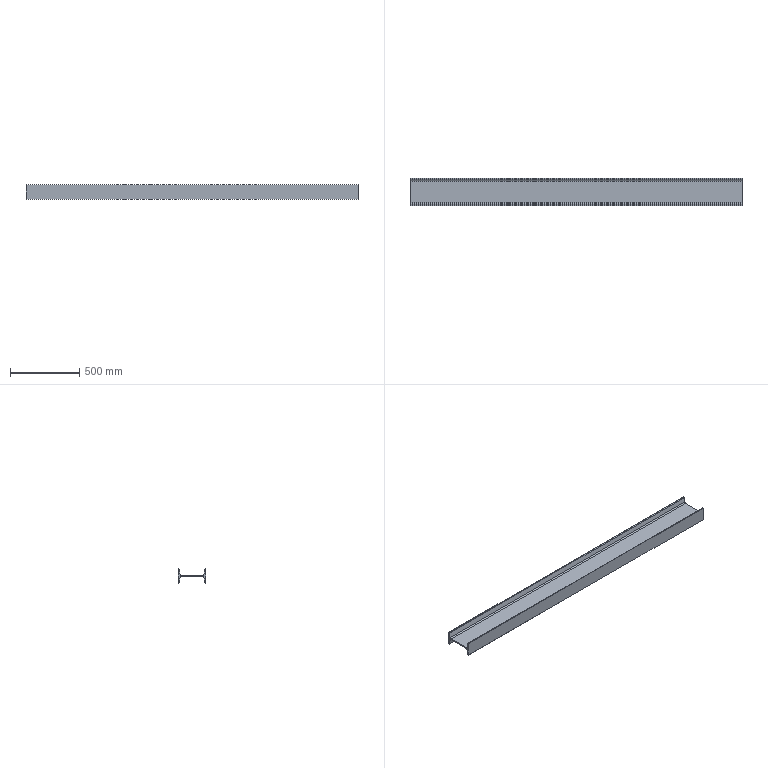Part | SolidWorks | features Fillet 2, Extrusion 1 | 1 solid | 22 faces | box 2400 x 200 x 102 mm | volume 9158318 mm3 | plane 14 | cylinder 8 | commonest cylinder face diameters 9 x4 18 x4
STEP:
#1=CARTESIAN_POINT('',(2400.,2.963,51.));
#2=VERTEX_POINT('',#1);
#3=CARTESIAN_POINT('',(2400.,0.,51.));
#4=VERTEX_POINT('',#3);
#5=CARTESIAN_POINT('',(2400.,6.775,51.));
#6=DIRECTION('',(0.,-1.,0.));
#7=VECTOR('',#6,1000.);
#8=LINE('',#5,#7);
#9=EDGE_CURVE('',#2,#4,#8,.T.);
#10=ORIENTED_EDGE('',*,*,#9,.F.);
#11=CARTESIAN_POINT('',(0.,2.963,51.));
#12=VERTEX_POINT('',#11);
#13=CARTESIAN_POINT('',(2400.,2.963,51.));
#14=DIRECTION('',(-1.,0.,0.));
#15=VECTOR('',#14,1000.);
#16=LINE('',#13,#15);
#17=EDGE_CURVE('',#2,#12,#16,.T.);
#18=ORIENTED_EDGE('',*,*,#17,.T.);
#19=CARTESIAN_POINT('',(0.,0.,51.));
#20=VERTEX_POINT('',#19);
#21=CARTESIAN_POINT('',(0.,6.775,51.));
#22=DIRECTION('',(0.,-1.,0.));
#23=VECTOR('',#22,1000.);
#24=LINE('',#21,#23);
#25=EDGE_CURVE('',#12,#20,#24,.T.);
#26=ORIENTED_EDGE('',*,*,#25,.T.);
#27=CARTESIAN_POINT('',(2400.,0.,51.));
#28=DIRECTION('',(-1.,0.,0.));
#29=VECTOR('',#28,1000.);
#30=LINE('',#27,#29);
#31=EDGE_CURVE('',#4,#20,#30,.T.);
#32=ORIENTED_EDGE('',*,*,#31,.F.);
#33=EDGE_LOOP('',(#10,#18,#26,#32));
#34=FACE_OUTER_BOUND('',#33,.T.);
#35=CARTESIAN_POINT('',(2400.,6.775,51.));
#36=DIRECTION('',(0.,0.,-1.));
#37=DIRECTION('',(-1.,0.,0.));
#38=AXIS2_PLACEMENT_3D('',#35,#36,#37);
#39=PLANE('',#38);
#40=ADVANCED_FACE('',(#34),#39,.F.);
#41=CARTESIAN_POINT('',(0.,0.,-51.));
#42=VERTEX_POINT('',#41);
#43=CARTESIAN_POINT('',(0.,0.,51.));
#44=DIRECTION('',(0.,0.,-1.));
#45=VECTOR('',#44,1000.);
#46=LINE('',#43,#45);
#47=EDGE_CURVE('',#20,#42,#46,.T.);
#48=ORIENTED_EDGE('',*,*,#47,.T.);
#49=CARTESIAN_POINT('',(2400.,0.,-51.));
#50=VERTEX_POINT('',#49);
#51=CARTESIAN_POINT('',(2400.,0.,-51.));
#52=DIRECTION('',(-1.,0.,0.));
#53=VECTOR('',#52,1000.);
#54=LINE('',#51,#53);
#55=EDGE_CURVE('',#50,#42,#54,.T.);
#56=ORIENTED_EDGE('',*,*,#55,.F.);
#57=CARTESIAN_POINT('',(2400.,0.,51.));
#58=DIRECTION('',(0.,0.,-1.));
#59=VECTOR('',#58,1000.);
#60=LINE('',#57,#59);
#61=EDGE_CURVE('',#4,#50,#60,.T.);
#62=ORIENTED_EDGE('',*,*,#61,.F.);
#63=ORIENTED_EDGE('',*,*,#31,.T.);
#64=EDGE_LOOP('',(#48,#56,#62,#63));
#65=FACE_OUTER_BOUND('',#64,.T.);
#66=CARTESIAN_POINT('',(2400.,0.,51.));
#67=DIRECTION('',(0.,1.,0.));
#68=DIRECTION('',(0.,0.,1.));
#69=AXIS2_PLACEMENT_3D('',#66,#67,#68);
#70=PLANE('',#69);
#71=ADVANCED_FACE('',(#65),#70,.F.);
#72=CARTESIAN_POINT('',(0.,2.963,-51.));
#73=VERTEX_POINT('',#72);
#74=CARTESIAN_POINT('',(0.,6.775,-51.));
#75=DIRECTION('',(0.,1.,0.));
#76=VECTOR('',#75,1000.);
#77=LINE('',#74,#76);
#78=EDGE_CURVE('',#42,#73,#77,.T.);
#79=ORIENTED_EDGE('',*,*,#78,.T.);
#80=CARTESIAN_POINT('',(2400.,2.963,-51.));
#81=VERTEX_POINT('',#80);
#82=CARTESIAN_POINT('',(2400.,2.963,-51.));
#83=DIRECTION('',(1.,0.,0.));
#84=VECTOR('',#83,1000.);
#85=LINE('',#82,#84);
#86=EDGE_CURVE('',#73,#81,#85,.T.);
#87=ORIENTED_EDGE('',*,*,#86,.T.);
#88=CARTESIAN_POINT('',(2400.,6.775,-51.));
#89=DIRECTION('',(0.,1.,0.));
#90=VECTOR('',#89,1000.);
#91=LINE('',#88,#90);
#92=EDGE_CURVE('',#50,#81,#91,.T.);
#93=ORIENTED_EDGE('',*,*,#92,.F.);
#94=ORIENTED_EDGE('',*,*,#55,.T.);
#95=EDGE_LOOP('',(#79,#87,#93,#94));
#96=FACE_OUTER_BOUND('',#95,.T.);
#97=CARTESIAN_POINT('',(2400.,6.775,-51.));
#98=DIRECTION('',(0.,0.,1.));
#99=DIRECTION('',(1.,0.,0.));
#100=AXIS2_PLACEMENT_3D('',#97,#98,#99);
#101=PLANE('',#100);
#102=ADVANCED_FACE('',(#96),#101,.F.);
#103=CARTESIAN_POINT('',(2400.,7.402,-47.24));
#104=VERTEX_POINT('',#103);
#105=CARTESIAN_POINT('',(2400.,13.272,-12.02));
#106=VERTEX_POINT('',#105);
#107=CARTESIAN_POINT('',(2400.,14.525,-4.5));
#108=DIRECTION('',(0.,0.1644,0.9864));
#109=VECTOR('',#108,1000.);
#110=LINE('',#107,#109);
#111=EDGE_CURVE('',#104,#106,#110,.T.);
#112=ORIENTED_EDGE('',*,*,#111,.F.);
#113=CARTESIAN_POINT('',(0.,7.402,-47.24));
#114=VERTEX_POINT('',#113);
#115=CARTESIAN_POINT('',(2400.,7.402,-47.24));
#116=DIRECTION('',(-1.,0.,0.));
#117=VECTOR('',#116,1000.);
#118=LINE('',#115,#117);
#119=EDGE_CURVE('',#104,#114,#118,.T.);
#120=ORIENTED_EDGE('',*,*,#119,.T.);
#121=CARTESIAN_POINT('',(0.,13.272,-12.02));
#122=VERTEX_POINT('',#121);
#123=CARTESIAN_POINT('',(0.,14.525,-4.5));
#124=DIRECTION('',(0.,0.1644,0.9864));
#125=VECTOR('',#124,1000.);
#126=LINE('',#123,#125);
#127=EDGE_CURVE('',#114,#122,#126,.T.);
#128=ORIENTED_EDGE('',*,*,#127,.T.);
#129=CARTESIAN_POINT('',(2400.,13.272,-12.02));
#130=DIRECTION('',(1.,0.,0.));
#131=VECTOR('',#130,1000.);
#132=LINE('',#129,#131);
#133=EDGE_CURVE('',#122,#106,#132,.T.);
#134=ORIENTED_EDGE('',*,*,#133,.T.);
#135=EDGE_LOOP('',(#112,#120,#128,#134));
#136=FACE_OUTER_BOUND('',#135,.T.);
#137=CARTESIAN_POINT('',(2400.,14.525,-4.5));
#138=DIRECTION('',(0.,-0.9864,0.1644));
#139=DIRECTION('',(0.,-0.1644,-0.9864));
#140=AXIS2_PLACEMENT_3D('',#137,#138,#139);
#141=PLANE('',#140);
#142=ADVANCED_FACE('',(#136),#141,.F.);
#143=CARTESIAN_POINT('',(0.,22.149,-4.5));
#144=VERTEX_POINT('',#143);
#145=CARTESIAN_POINT('',(0.,177.851,-4.5));
#146=VERTEX_POINT('',#145);
#147=CARTESIAN_POINT('',(0.,185.475,-4.5));
#148=DIRECTION('',(0.,1.,0.));
#149=VECTOR('',#148,1000.);
#150=LINE('',#147,#149);
#151=EDGE_CURVE('',#144,#146,#150,.T.);
#152=ORIENTED_EDGE('',*,*,#151,.T.);
#153=CARTESIAN_POINT('',(2400.,177.851,-4.5));
#154=VERTEX_POINT('',#153);
#155=CARTESIAN_POINT('',(2400.,177.851,-4.5));
#156=DIRECTION('',(1.,0.,0.));
#157=VECTOR('',#156,1000.);
#158=LINE('',#155,#157);
#159=EDGE_CURVE('',#146,#154,#158,.T.);
#160=ORIENTED_EDGE('',*,*,#159,.T.);
#161=CARTESIAN_POINT('',(2400.,22.149,-4.5));
#162=VERTEX_POINT('',#161);
#163=CARTESIAN_POINT('',(2400.,185.475,-4.5));
#164=DIRECTION('',(0.,1.,0.));
#165=VECTOR('',#164,1000.);
#166=LINE('',#163,#165);
#167=EDGE_CURVE('',#162,#154,#166,.T.);
#168=ORIENTED_EDGE('',*,*,#167,.F.);
#169=CARTESIAN_POINT('',(0.,22.149,-4.5));
#170=DIRECTION('',(-1.,0.,0.));
#171=VECTOR('',#170,1000.);
#172=LINE('',#169,#171);
#173=EDGE_CURVE('',#162,#144,#172,.T.);
#174=ORIENTED_EDGE('',*,*,#173,.T.);
#175=EDGE_LOOP('',(#152,#160,#168,#174));
#176=FACE_OUTER_BOUND('',#175,.T.);
#177=CARTESIAN_POINT('',(2400.,185.475,-4.5));
#178=DIRECTION('',(0.,0.,1.));
#179=DIRECTION('',(0.,-1.,0.));
#180=AXIS2_PLACEMENT_3D('',#177,#178,#179);
#181=PLANE('',#180);
#182=ADVANCED_FACE('',(#176),#181,.F.);
#183=CARTESIAN_POINT('',(0.,186.728,-12.02));
#184=VERTEX_POINT('',#183);
#185=CARTESIAN_POINT('',(0.,192.598,-47.24));
#186=VERTEX_POINT('',#185);
#187=CARTESIAN_POINT('',(0.,193.225,-51.));
#188=DIRECTION('',(0.,0.1644,-0.9864));
#189=VECTOR('',#188,1000.);
#190=LINE('',#187,#189);
#191=EDGE_CURVE('',#184,#186,#190,.T.);
#192=ORIENTED_EDGE('',*,*,#191,.T.);
#193=CARTESIAN_POINT('',(2400.,192.598,-47.24));
#194=VERTEX_POINT('',#193);
#195=CARTESIAN_POINT('',(2400.,192.598,-47.24));
#196=DIRECTION('',(1.,0.,0.));
#197=VECTOR('',#196,1000.);
#198=LINE('',#195,#197);
#199=EDGE_CURVE('',#186,#194,#198,.T.);
#200=ORIENTED_EDGE('',*,*,#199,.T.);
#201=CARTESIAN_POINT('',(2400.,186.728,-12.02));
#202=VERTEX_POINT('',#201);
#203=CARTESIAN_POINT('',(2400.,193.225,-51.));
#204=DIRECTION('',(0.,0.1644,-0.9864));
#205=VECTOR('',#204,1000.);
#206=LINE('',#203,#205);
#207=EDGE_CURVE('',#202,#194,#206,.T.);
#208=ORIENTED_EDGE('',*,*,#207,.F.);
#209=CARTESIAN_POINT('',(0.,186.728,-12.02));
#210=DIRECTION('',(-1.,0.,0.));
#211=VECTOR('',#210,1000.);
#212=LINE('',#209,#211);
#213=EDGE_CURVE('',#202,#184,#212,.T.);
#214=ORIENTED_EDGE('',*,*,#213,.T.);
#215=EDGE_LOOP('',(#192,#200,#208,#214));
#216=FACE_OUTER_BOUND('',#215,.T.);
#217=CARTESIAN_POINT('',(2400.,193.225,-51.));
#218=DIRECTION('',(0.,0.9864,0.1644));
#219=DIRECTION('',(0.,-0.1644,0.9864));
#220=AXIS2_PLACEMENT_3D('',#217,#218,#219);
#221=PLANE('',#220);
#222=ADVANCED_FACE('',(#216),#221,.F.);
#223=CARTESIAN_POINT('',(2400.,197.037,-51.));
#224=VERTEX_POINT('',#223);
#225=CARTESIAN_POINT('',(2400.,200.,-51.));
#226=VERTEX_POINT('',#225);
#227=CARTESIAN_POINT('',(2400.,200.,-51.));
#228=DIRECTION('',(0.,1.,0.));
#229=VECTOR('',#228,1000.);
#230=LINE('',#227,#229);
#231=EDGE_CURVE('',#224,#226,#230,.T.);
#232=ORIENTED_EDGE('',*,*,#231,.F.);
#233=CARTESIAN_POINT('',(0.,197.037,-51.));
#234=VERTEX_POINT('',#233);
#235=CARTESIAN_POINT('',(2400.,197.037,-51.));
#236=DIRECTION('',(-1.,0.,0.));
#237=VECTOR('',#236,1000.);
#238=LINE('',#235,#237);
#239=EDGE_CURVE('',#224,#234,#238,.T.);
#240=ORIENTED_EDGE('',*,*,#239,.T.);
#241=CARTESIAN_POINT('',(0.,200.,-51.));
#242=VERTEX_POINT('',#241);
#243=CARTESIAN_POINT('',(0.,200.,-51.));
#244=DIRECTION('',(0.,1.,0.));
#245=VECTOR('',#244,1000.);
#246=LINE('',#243,#245);
#247=EDGE_CURVE('',#234,#242,#246,.T.);
#248=ORIENTED_EDGE('',*,*,#247,.T.);
#249=CARTESIAN_POINT('',(2400.,200.,-51.));
#250=DIRECTION('',(-1.,0.,0.));
#251=VECTOR('',#250,1000.);
#252=LINE('',#249,#251);
#253=EDGE_CURVE('',#226,#242,#252,.T.);
#254=ORIENTED_EDGE('',*,*,#253,.F.);
#255=EDGE_LOOP('',(#232,#240,#248,#254));
#256=FACE_OUTER_BOUND('',#255,.T.);
#257=CARTESIAN_POINT('',(2400.,200.,-51.));
#258=DIRECTION('',(0.,0.,1.));
#259=DIRECTION('',(0.,-1.,0.));
#260=AXIS2_PLACEMENT_3D('',#257,#258,#259);
#261=PLANE('',#260);
#262=ADVANCED_FACE('',(#256),#261,.F.);
#263=CARTESIAN_POINT('',(0.,200.,51.));
#264=VERTEX_POINT('',#263);
#265=CARTESIAN_POINT('',(0.,200.,51.));
#266=DIRECTION('',(0.,0.,1.));
#267=VECTOR('',#266,1000.);
#268=LINE('',#265,#267);
#269=EDGE_CURVE('',#242,#264,#268,.T.);
#270=ORIENTED_EDGE('',*,*,#269,.T.);
#271=CARTESIAN_POINT('',(2400.,200.,51.));
#272=VERTEX_POINT('',#271);
#273=CARTESIAN_POINT('',(2400.,200.,51.));
#274=DIRECTION('',(-1.,0.,0.));
#275=VECTOR('',#274,1000.);
#276=LINE('',#273,#275);
#277=EDGE_CURVE('',#272,#264,#276,.T.);
#278=ORIENTED_EDGE('',*,*,#277,.F.);
#279=CARTESIAN_POINT('',(2400.,200.,51.));
#280=DIRECTION('',(0.,0.,1.));
#281=VECTOR('',#280,1000.);
#282=LINE('',#279,#281);
#283=EDGE_CURVE('',#226,#272,#282,.T.);
#284=ORIENTED_EDGE('',*,*,#283,.F.);
#285=ORIENTED_EDGE('',*,*,#253,.T.);
#286=EDGE_LOOP('',(#270,#278,#284,#285));
#287=FACE_OUTER_BOUND('',#286,.T.);
#288=CARTESIAN_POINT('',(2400.,200.,51.));
#289=DIRECTION('',(0.,-1.,0.));
#290=DIRECTION('',(0.,0.,-1.));
#291=AXIS2_PLACEMENT_3D('',#288,#289,#290);
#292=PLANE('',#291);
#293=ADVANCED_FACE('',(#287),#292,.F.);
#294=CARTESIAN_POINT('',(0.,197.037,51.));
#295=VERTEX_POINT('',#294);
#296=CARTESIAN_POINT('',(0.,200.,51.));
#297=DIRECTION('',(0.,-1.,0.));
#298=VECTOR('',#297,1000.);
#299=LINE('',#296,#298);
#300=EDGE_CURVE('',#264,#295,#299,.T.);
#301=ORIENTED_EDGE('',*,*,#300,.T.);
#302=CARTESIAN_POINT('',(2400.,197.037,51.));
#303=VERTEX_POINT('',#302);
#304=CARTESIAN_POINT('',(2400.,197.037,51.));
#305=DIRECTION('',(1.,0.,0.));
#306=VECTOR('',#305,1000.);
#307=LINE('',#304,#306);
#308=EDGE_CURVE('',#295,#303,#307,.T.);
#309=ORIENTED_EDGE('',*,*,#308,.T.);
#310=CARTESIAN_POINT('',(2400.,200.,51.));
#311=DIRECTION('',(0.,-1.,0.));
#312=VECTOR('',#311,1000.);
#313=LINE('',#310,#312);
#314=EDGE_CURVE('',#272,#303,#313,.T.);
#315=ORIENTED_EDGE('',*,*,#314,.F.);
#316=ORIENTED_EDGE('',*,*,#277,.T.);
#317=EDGE_LOOP('',(#301,#309,#315,#316));
#318=FACE_OUTER_BOUND('',#317,.T.);
#319=CARTESIAN_POINT('',(2400.,200.,51.));
#320=DIRECTION('',(0.,0.,-1.));
#321=DIRECTION('',(0.,1.,0.));
#322=AXIS2_PLACEMENT_3D('',#319,#320,#321);
#323=PLANE('',#322);
#324=ADVANCED_FACE('',(#318),#323,.F.);
#325=CARTESIAN_POINT('',(2400.,192.598,47.24));
#326=VERTEX_POINT('',#325);
#327=CARTESIAN_POINT('',(2400.,186.728,12.02));
#328=VERTEX_POINT('',#327);
#329=CARTESIAN_POINT('',(2400.,193.225,51.));
#330=DIRECTION('',(0.,-0.1644,-0.9864));
#331=VECTOR('',#330,1000.);
#332=LINE('',#329,#331);
#333=EDGE_CURVE('',#326,#328,#332,.T.);
#334=ORIENTED_EDGE('',*,*,#333,.F.);
#335=CARTESIAN_POINT('',(0.,192.598,47.24));
#336=VERTEX_POINT('',#335);
#337=CARTESIAN_POINT('',(2400.,192.598,47.24));
#338=DIRECTION('',(-1.,0.,0.));
#339=VECTOR('',#338,1000.);
#340=LINE('',#337,#339);
#341=EDGE_CURVE('',#326,#336,#340,.T.);
#342=ORIENTED_EDGE('',*,*,#341,.T.);
#343=CARTESIAN_POINT('',(0.,186.728,12.02));
#344=VERTEX_POINT('',#343);
#345=CARTESIAN_POINT('',(0.,193.225,51.));
#346=DIRECTION('',(0.,-0.1644,-0.9864));
#347=VECTOR('',#346,1000.);
#348=LINE('',#345,#347);
#349=EDGE_CURVE('',#336,#344,#348,.T.);
#350=ORIENTED_EDGE('',*,*,#349,.T.);
#351=CARTESIAN_POINT('',(2400.,186.728,12.02));
#352=DIRECTION('',(1.,0.,0.));
#353=VECTOR('',#352,1000.);
#354=LINE('',#351,#353);
#355=EDGE_CURVE('',#344,#328,#354,.T.);
#356=ORIENTED_EDGE('',*,*,#355,.T.);
#357=EDGE_LOOP('',(#334,#342,#350,#356));
#358=FACE_OUTER_BOUND('',#357,.T.);
#359=CARTESIAN_POINT('',(2400.,193.225,51.));
#360=DIRECTION('',(0.,0.9864,-0.1644));
#361=DIRECTION('',(0.,0.1644,0.9864));
#362=AXIS2_PLACEMENT_3D('',#359,#360,#361);
#363=PLANE('',#362);
#364=ADVANCED_FACE('',(#358),#363,.F.);
#365=CARTESIAN_POINT('',(0.,177.851,4.5));
#366=VERTEX_POINT('',#365);
#367=CARTESIAN_POINT('',(0.,22.149,4.5));
#368=VERTEX_POINT('',#367);
#369=CARTESIAN_POINT('',(0.,185.475,4.5));
#370=DIRECTION('',(0.,-1.,0.));
#371=VECTOR('',#370,1000.);
#372=LINE('',#369,#371);
#373=EDGE_CURVE('',#366,#368,#372,.T.);
#374=ORIENTED_EDGE('',*,*,#373,.T.);
#375=CARTESIAN_POINT('',(2400.,22.149,4.5));
#376=VERTEX_POINT('',#375);
#377=CARTESIAN_POINT('',(2400.,22.149,4.5));
#378=DIRECTION('',(1.,0.,0.));
#379=VECTOR('',#378,1000.);
#380=LINE('',#377,#379);
#381=EDGE_CURVE('',#368,#376,#380,.T.);
#382=ORIENTED_EDGE('',*,*,#381,.T.);
#383=CARTESIAN_POINT('',(2400.,177.851,4.5));
#384=VERTEX_POINT('',#383);
#385=CARTESIAN_POINT('',(2400.,185.475,4.5));
#386=DIRECTION('',(0.,-1.,0.));
#387=VECTOR('',#386,1000.);
#388=LINE('',#385,#387);
#389=EDGE_CURVE('',#384,#376,#388,.T.);
#390=ORIENTED_EDGE('',*,*,#389,.F.);
#391=CARTESIAN_POINT('',(0.,177.851,4.5));
#392=DIRECTION('',(-1.,0.,0.));
#393=VECTOR('',#392,1000.);
#394=LINE('',#391,#393);
#395=EDGE_CURVE('',#384,#366,#394,.T.);
#396=ORIENTED_EDGE('',*,*,#395,.T.);
#397=EDGE_LOOP('',(#374,#382,#390,#396));
#398=FACE_OUTER_BOUND('',#397,.T.);
#399=CARTESIAN_POINT('',(2400.,185.475,4.5));
#400=DIRECTION('',(0.,0.,-1.));
#401=DIRECTION('',(0.,1.,0.));
#402=AXIS2_PLACEMENT_3D('',#399,#400,#401);
#403=PLANE('',#402);
#404=ADVANCED_FACE('',(#398),#403,.F.);
#405=CARTESIAN_POINT('',(0.,13.272,12.02));
#406=VERTEX_POINT('',#405);
#407=CARTESIAN_POINT('',(0.,7.402,47.24));
#408=VERTEX_POINT('',#407);
#409=CARTESIAN_POINT('',(0.,14.525,4.5));
#410=DIRECTION('',(0.,-0.1644,0.9864));
#411=VECTOR('',#410,1000.);
#412=LINE('',#409,#411);
#413=EDGE_CURVE('',#406,#408,#412,.T.);
#414=ORIENTED_EDGE('',*,*,#413,.T.);
#415=CARTESIAN_POINT('',(2400.,7.402,47.24));
#416=VERTEX_POINT('',#415);
#417=CARTESIAN_POINT('',(2400.,7.402,47.24));
#418=DIRECTION('',(1.,0.,0.));
#419=VECTOR('',#418,1000.);
#420=LINE('',#417,#419);
#421=EDGE_CURVE('',#408,#416,#420,.T.);
#422=ORIENTED_EDGE('',*,*,#421,.T.);
#423=CARTESIAN_POINT('',(2400.,13.272,12.02));
#424=VERTEX_POINT('',#423);
#425=CARTESIAN_POINT('',(2400.,14.525,4.5));
#426=DIRECTION('',(0.,-0.1644,0.9864));
#427=VECTOR('',#426,1000.);
#428=LINE('',#425,#427);
#429=EDGE_CURVE('',#424,#416,#428,.T.);
#430=ORIENTED_EDGE('',*,*,#429,.F.);
#431=CARTESIAN_POINT('',(0.,13.272,12.02));
#432=DIRECTION('',(-1.,0.,0.));
#433=VECTOR('',#432,1000.);
#434=LINE('',#431,#433);
#435=EDGE_CURVE('',#424,#406,#434,.T.);
#436=ORIENTED_EDGE('',*,*,#435,.T.);
#437=EDGE_LOOP('',(#414,#422,#430,#436));
#438=FACE_OUTER_BOUND('',#437,.T.);
#439=CARTESIAN_POINT('',(2400.,14.525,4.5));
#440=DIRECTION('',(0.,-0.9864,-0.1644));
#441=DIRECTION('',(0.,0.1644,-0.9864));
#442=AXIS2_PLACEMENT_3D('',#439,#440,#441);
#443=PLANE('',#442);
#444=ADVANCED_FACE('',(#438),#443,.F.);
#445=ORIENTED_EDGE('',*,*,#314,.T.);
#446=CARTESIAN_POINT('',(2400.,197.037,46.5));
#447=DIRECTION('',(1.,0.,0.));
#448=DIRECTION('',(0.,0.,-1.));
#449=AXIS2_PLACEMENT_3D('',#446,#447,#448);
#450=CIRCLE('',#449,4.5);
#451=EDGE_CURVE('',#303,#326,#450,.T.);
#452=ORIENTED_EDGE('',*,*,#451,.T.);
#453=ORIENTED_EDGE('',*,*,#333,.T.);
#454=CARTESIAN_POINT('',(2400.,177.851,13.5));
#455=DIRECTION('',(-1.,0.,0.));
#456=DIRECTION('',(0.,0.,-1.));
#457=AXIS2_PLACEMENT_3D('',#454,#455,#456);
#458=CIRCLE('',#457,9.);
#459=EDGE_CURVE('',#328,#384,#458,.T.);
#460=ORIENTED_EDGE('',*,*,#459,.T.);
#461=ORIENTED_EDGE('',*,*,#389,.T.);
#462=CARTESIAN_POINT('',(2400.,22.149,13.5));
#463=DIRECTION('',(-1.,0.,0.));
#464=DIRECTION('',(0.,0.,-1.));
#465=AXIS2_PLACEMENT_3D('',#462,#463,#464);
#466=CIRCLE('',#465,9.);
#467=EDGE_CURVE('',#376,#424,#466,.T.);
#468=ORIENTED_EDGE('',*,*,#467,.T.);
#469=ORIENTED_EDGE('',*,*,#429,.T.);
#470=CARTESIAN_POINT('',(2400.,2.963,46.5));
#471=DIRECTION('',(1.,0.,0.));
#472=DIRECTION('',(0.,0.,-1.));
#473=AXIS2_PLACEMENT_3D('',#470,#471,#472);
#474=CIRCLE('',#473,4.5);
#475=EDGE_CURVE('',#416,#2,#474,.T.);
#476=ORIENTED_EDGE('',*,*,#475,.T.);
#477=ORIENTED_EDGE('',*,*,#9,.T.);
#478=ORIENTED_EDGE('',*,*,#61,.T.);
#479=ORIENTED_EDGE('',*,*,#92,.T.);
#480=CARTESIAN_POINT('',(2400.,2.963,-46.5));
#481=DIRECTION('',(1.,0.,0.));
#482=DIRECTION('',(0.,0.,-1.));
#483=AXIS2_PLACEMENT_3D('',#480,#481,#482);
#484=CIRCLE('',#483,4.5);
#485=EDGE_CURVE('',#81,#104,#484,.T.);
#486=ORIENTED_EDGE('',*,*,#485,.T.);
#487=ORIENTED_EDGE('',*,*,#111,.T.);
#488=CARTESIAN_POINT('',(2400.,22.149,-13.5));
#489=DIRECTION('',(-1.,0.,0.));
#490=DIRECTION('',(0.,0.,-1.));
#491=AXIS2_PLACEMENT_3D('',#488,#489,#490);
#492=CIRCLE('',#491,9.);
#493=EDGE_CURVE('',#106,#162,#492,.T.);
#494=ORIENTED_EDGE('',*,*,#493,.T.);
#495=ORIENTED_EDGE('',*,*,#167,.T.);
#496=CARTESIAN_POINT('',(2400.,177.851,-13.5));
#497=DIRECTION('',(-1.,0.,0.));
#498=DIRECTION('',(0.,0.,-1.));
#499=AXIS2_PLACEMENT_3D('',#496,#497,#498);
#500=CIRCLE('',#499,9.);
#501=EDGE_CURVE('',#154,#202,#500,.T.);
#502=ORIENTED_EDGE('',*,*,#501,.T.);
#503=ORIENTED_EDGE('',*,*,#207,.T.);
#504=CARTESIAN_POINT('',(2400.,197.037,-46.5));
#505=DIRECTION('',(1.,0.,0.));
#506=DIRECTION('',(0.,0.,-1.));
#507=AXIS2_PLACEMENT_3D('',#504,#505,#506);
#508=CIRCLE('',#507,4.5);
#509=EDGE_CURVE('',#194,#224,#508,.T.);
#510=ORIENTED_EDGE('',*,*,#509,.T.);
#511=ORIENTED_EDGE('',*,*,#231,.T.);
#512=ORIENTED_EDGE('',*,*,#283,.T.);
#513=EDGE_LOOP('',(#445,#452,#453,#460,#461,#468,#469,#476,#477,#478,#479,#486,#487,#494,#495,#502,#503,#510,#511,#512));
#514=FACE_OUTER_BOUND('',#513,.T.);
#515=CARTESIAN_POINT('',(2400.,200.,51.));
#516=DIRECTION('',(1.,0.,0.));
#517=DIRECTION('',(0.,0.,-1.));
#518=AXIS2_PLACEMENT_3D('',#515,#516,#517);
#519=PLANE('',#518);
#520=ADVANCED_FACE('',(#514),#519,.T.);
#521=ORIENTED_EDGE('',*,*,#349,.F.);
#522=CARTESIAN_POINT('',(0.,197.037,46.5));
#523=DIRECTION('',(-1.,0.,0.));
#524=DIRECTION('',(0.,0.,-1.));
#525=AXIS2_PLACEMENT_3D('',#522,#523,#524);
#526=CIRCLE('',#525,4.5);
#527=EDGE_CURVE('',#336,#295,#526,.T.);
#528=ORIENTED_EDGE('',*,*,#527,.T.);
#529=ORIENTED_EDGE('',*,*,#300,.F.);
#530=ORIENTED_EDGE('',*,*,#269,.F.);
#531=ORIENTED_EDGE('',*,*,#247,.F.);
#532=CARTESIAN_POINT('',(0.,197.037,-46.5));
#533=DIRECTION('',(-1.,0.,0.));
#534=DIRECTION('',(0.,0.,-1.));
#535=AXIS2_PLACEMENT_3D('',#532,#533,#534);
#536=CIRCLE('',#535,4.5);
#537=EDGE_CURVE('',#234,#186,#536,.T.);
#538=ORIENTED_EDGE('',*,*,#537,.T.);
#539=ORIENTED_EDGE('',*,*,#191,.F.);
#540=CARTESIAN_POINT('',(0.,177.851,-13.5));
#541=DIRECTION('',(1.,0.,0.));
#542=DIRECTION('',(0.,0.,-1.));
#543=AXIS2_PLACEMENT_3D('',#540,#541,#542);
#544=CIRCLE('',#543,9.);
#545=EDGE_CURVE('',#184,#146,#544,.T.);
#546=ORIENTED_EDGE('',*,*,#545,.T.);
#547=ORIENTED_EDGE('',*,*,#151,.F.);
#548=CARTESIAN_POINT('',(0.,22.149,-13.5));
#549=DIRECTION('',(1.,0.,0.));
#550=DIRECTION('',(0.,0.,-1.));
#551=AXIS2_PLACEMENT_3D('',#548,#549,#550);
#552=CIRCLE('',#551,9.);
#553=EDGE_CURVE('',#144,#122,#552,.T.);
#554=ORIENTED_EDGE('',*,*,#553,.T.);
#555=ORIENTED_EDGE('',*,*,#127,.F.);
#556=CARTESIAN_POINT('',(0.,2.963,-46.5));
#557=DIRECTION('',(-1.,0.,0.));
#558=DIRECTION('',(0.,0.,-1.));
#559=AXIS2_PLACEMENT_3D('',#556,#557,#558);
#560=CIRCLE('',#559,4.5);
#561=EDGE_CURVE('',#114,#73,#560,.T.);
#562=ORIENTED_EDGE('',*,*,#561,.T.);
#563=ORIENTED_EDGE('',*,*,#78,.F.);
#564=ORIENTED_EDGE('',*,*,#47,.F.);
#565=ORIENTED_EDGE('',*,*,#25,.F.);
#566=CARTESIAN_POINT('',(0.,2.963,46.5));
#567=DIRECTION('',(-1.,0.,0.));
#568=DIRECTION('',(0.,0.,-1.));
#569=AXIS2_PLACEMENT_3D('',#566,#567,#568);
#570=CIRCLE('',#569,4.5);
#571=EDGE_CURVE('',#12,#408,#570,.T.);
#572=ORIENTED_EDGE('',*,*,#571,.T.);
#573=ORIENTED_EDGE('',*,*,#413,.F.);
#574=CARTESIAN_POINT('',(0.,22.149,13.5));
#575=DIRECTION('',(1.,0.,0.));
#576=DIRECTION('',(0.,0.,-1.));
#577=AXIS2_PLACEMENT_3D('',#574,#575,#576);
#578=CIRCLE('',#577,9.);
#579=EDGE_CURVE('',#406,#368,#578,.T.);
#580=ORIENTED_EDGE('',*,*,#579,.T.);
#581=ORIENTED_EDGE('',*,*,#373,.F.);
#582=CARTESIAN_POINT('',(0.,177.851,13.5));
#583=DIRECTION('',(1.,0.,0.));
#584=DIRECTION('',(0.,0.,-1.));
#585=AXIS2_PLACEMENT_3D('',#582,#583,#584);
#586=CIRCLE('',#585,9.);
#587=EDGE_CURVE('',#366,#344,#586,.T.);
#588=ORIENTED_EDGE('',*,*,#587,.T.);
#589=EDGE_LOOP('',(#521,#528,#529,#530,#531,#538,#539,#546,#547,#554,#555,#562,#563,#564,#565,#572,#573,#580,#581,#588));
#590=FACE_OUTER_BOUND('',#589,.T.);
#591=CARTESIAN_POINT('',(0.,200.,51.));
#592=DIRECTION('',(1.,0.,0.));
#593=DIRECTION('',(0.,0.,-1.));
#594=AXIS2_PLACEMENT_3D('',#591,#592,#593);
#595=PLANE('',#594);
#596=ADVANCED_FACE('',(#590),#595,.F.);
#597=ORIENTED_EDGE('',*,*,#501,.F.);
#598=ORIENTED_EDGE('',*,*,#159,.F.);
#599=ORIENTED_EDGE('',*,*,#545,.F.);
#600=ORIENTED_EDGE('',*,*,#213,.F.);
#601=EDGE_LOOP('',(#597,#598,#599,#600));
#602=FACE_OUTER_BOUND('',#601,.T.);
#603=CARTESIAN_POINT('',(2400.,177.851,-13.5));
#604=DIRECTION('',(1.,0.,0.));
#605=DIRECTION('',(0.,0.,-1.));
#606=AXIS2_PLACEMENT_3D('',#603,#604,#605);
#607=CYLINDRICAL_SURFACE('',#606,9.);
#608=ADVANCED_FACE('',(#602),#607,.F.);
#609=ORIENTED_EDGE('',*,*,#493,.F.);
#610=ORIENTED_EDGE('',*,*,#133,.F.);
#611=ORIENTED_EDGE('',*,*,#553,.F.);
#612=ORIENTED_EDGE('',*,*,#173,.F.);
#613=EDGE_LOOP('',(#609,#610,#611,#612));
#614=FACE_OUTER_BOUND('',#613,.T.);
#615=CARTESIAN_POINT('',(2400.,22.149,-13.5));
#616=DIRECTION('',(1.,0.,0.));
#617=DIRECTION('',(0.,0.,-1.));
#618=AXIS2_PLACEMENT_3D('',#615,#616,#617);
#619=CYLINDRICAL_SURFACE('',#618,9.);
#620=ADVANCED_FACE('',(#614),#619,.F.);
#621=ORIENTED_EDGE('',*,*,#467,.F.);
#622=ORIENTED_EDGE('',*,*,#381,.F.);
#623=ORIENTED_EDGE('',*,*,#579,.F.);
#624=ORIENTED_EDGE('',*,*,#435,.F.);
#625=EDGE_LOOP('',(#621,#622,#623,#624));
#626=FACE_OUTER_BOUND('',#625,.T.);
#627=CARTESIAN_POINT('',(2400.,22.149,13.5));
#628=DIRECTION('',(1.,0.,0.));
#629=DIRECTION('',(0.,0.,-1.));
#630=AXIS2_PLACEMENT_3D('',#627,#628,#629);
#631=CYLINDRICAL_SURFACE('',#630,9.);
#632=ADVANCED_FACE('',(#626),#631,.F.);
#633=ORIENTED_EDGE('',*,*,#459,.F.);
#634=ORIENTED_EDGE('',*,*,#355,.F.);
#635=ORIENTED_EDGE('',*,*,#587,.F.);
#636=ORIENTED_EDGE('',*,*,#395,.F.);
#637=EDGE_LOOP('',(#633,#634,#635,#636));
#638=FACE_OUTER_BOUND('',#637,.T.);
#639=CARTESIAN_POINT('',(2400.,177.851,13.5));
#640=DIRECTION('',(1.,0.,0.));
#641=DIRECTION('',(0.,0.,-1.));
#642=AXIS2_PLACEMENT_3D('',#639,#640,#641);
#643=CYLINDRICAL_SURFACE('',#642,9.);
#644=ADVANCED_FACE('',(#638),#643,.F.);
#645=ORIENTED_EDGE('',*,*,#451,.F.);
#646=ORIENTED_EDGE('',*,*,#308,.F.);
#647=ORIENTED_EDGE('',*,*,#527,.F.);
#648=ORIENTED_EDGE('',*,*,#341,.F.);
#649=EDGE_LOOP('',(#645,#646,#647,#648));
#650=FACE_OUTER_BOUND('',#649,.T.);
#651=CARTESIAN_POINT('',(2400.,197.037,46.5));
#652=DIRECTION('',(-1.,0.,0.));
#653=DIRECTION('',(0.,0.,1.));
#654=AXIS2_PLACEMENT_3D('',#651,#652,#653);
#655=CYLINDRICAL_SURFACE('',#654,4.5);
#656=ADVANCED_FACE('',(#650),#655,.T.);
#657=ORIENTED_EDGE('',*,*,#475,.F.);
#658=ORIENTED_EDGE('',*,*,#421,.F.);
#659=ORIENTED_EDGE('',*,*,#571,.F.);
#660=ORIENTED_EDGE('',*,*,#17,.F.);
#661=EDGE_LOOP('',(#657,#658,#659,#660));
#662=FACE_OUTER_BOUND('',#661,.T.);
#663=CARTESIAN_POINT('',(2400.,2.963,46.5));
#664=DIRECTION('',(-1.,0.,0.));
#665=DIRECTION('',(0.,0.,1.));
#666=AXIS2_PLACEMENT_3D('',#663,#664,#665);
#667=CYLINDRICAL_SURFACE('',#666,4.5);
#668=ADVANCED_FACE('',(#662),#667,.T.);
#669=ORIENTED_EDGE('',*,*,#485,.F.);
#670=ORIENTED_EDGE('',*,*,#86,.F.);
#671=ORIENTED_EDGE('',*,*,#561,.F.);
#672=ORIENTED_EDGE('',*,*,#119,.F.);
#673=EDGE_LOOP('',(#669,#670,#671,#672));
#674=FACE_OUTER_BOUND('',#673,.T.);
#675=CARTESIAN_POINT('',(2400.,2.963,-46.5));
#676=DIRECTION('',(-1.,0.,0.));
#677=DIRECTION('',(0.,0.,1.));
#678=AXIS2_PLACEMENT_3D('',#675,#676,#677);
#679=CYLINDRICAL_SURFACE('',#678,4.5);
#680=ADVANCED_FACE('',(#674),#679,.T.);
#681=ORIENTED_EDGE('',*,*,#509,.F.);
#682=ORIENTED_EDGE('',*,*,#199,.F.);
#683=ORIENTED_EDGE('',*,*,#537,.F.);
#684=ORIENTED_EDGE('',*,*,#239,.F.);
#685=EDGE_LOOP('',(#681,#682,#683,#684));
#686=FACE_OUTER_BOUND('',#685,.T.);
#687=CARTESIAN_POINT('',(2400.,197.037,-46.5));
#688=DIRECTION('',(-1.,0.,0.));
#689=DIRECTION('',(0.,0.,1.));
#690=AXIS2_PLACEMENT_3D('',#687,#688,#689);
#691=CYLINDRICAL_SURFACE('',#690,4.5);
#692=ADVANCED_FACE('',(#686),#691,.T.);
#693=CLOSED_SHELL('',(#40,#71,#102,#142,#182,#222,#262,#293,#324,#364,#404,#444,#520,#596,#608,#620,#632,#644,#656,#668,#680,#692));
#694=MANIFOLD_SOLID_BREP('',#693);
#695=CARTESIAN_POINT('',(0.,0.,0.));
#696=DIRECTION('',(0.,0.,1.));
#697=DIRECTION('',(1.,0.,0.));
#698=AXIS2_PLACEMENT_3D('',#695,#696,#697);
#699=(LENGTH_UNIT()NAMED_UNIT(*)SI_UNIT(.MILLI.,.METRE.));
#700=UNCERTAINTY_MEASURE_WITH_UNIT(LENGTH_MEASURE(0.00001),#699,'','');
#701=(NAMED_UNIT(*)PLANE_ANGLE_UNIT()SI_UNIT($,.RADIAN.));
#702=(NAMED_UNIT(*)SI_UNIT($,.STERADIAN.)SOLID_ANGLE_UNIT());
#703=(GEOMETRIC_REPRESENTATION_CONTEXT(3)GLOBAL_UNCERTAINTY_ASSIGNED_CONTEXT((#700))GLOBAL_UNIT_ASSIGNED_CONTEXT((#699,#701,#702))REPRESENTATION_CONTEXT('',''));
#704=ADVANCED_BREP_SHAPE_REPRESENTATION('',(#694,#698),#703);